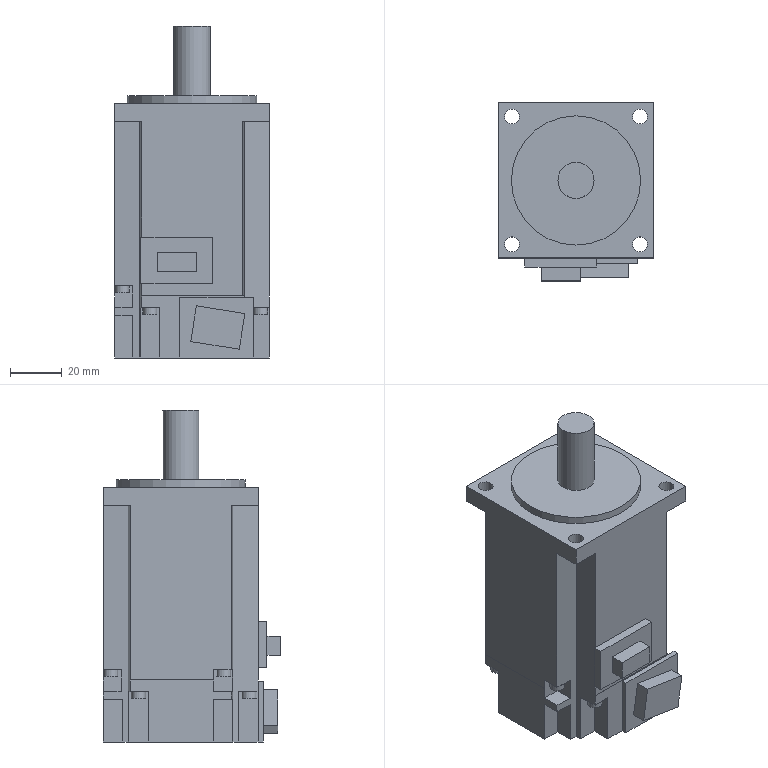Part | NX | 1 solid | 104 faces | box 60 x 68.8 x 128.5 mm | volume 323786 mm3 | plane 91 | cylinder 13 | commonest cylinder face diameters 5.5 x7 5.8 x4 14 x1 50 x1